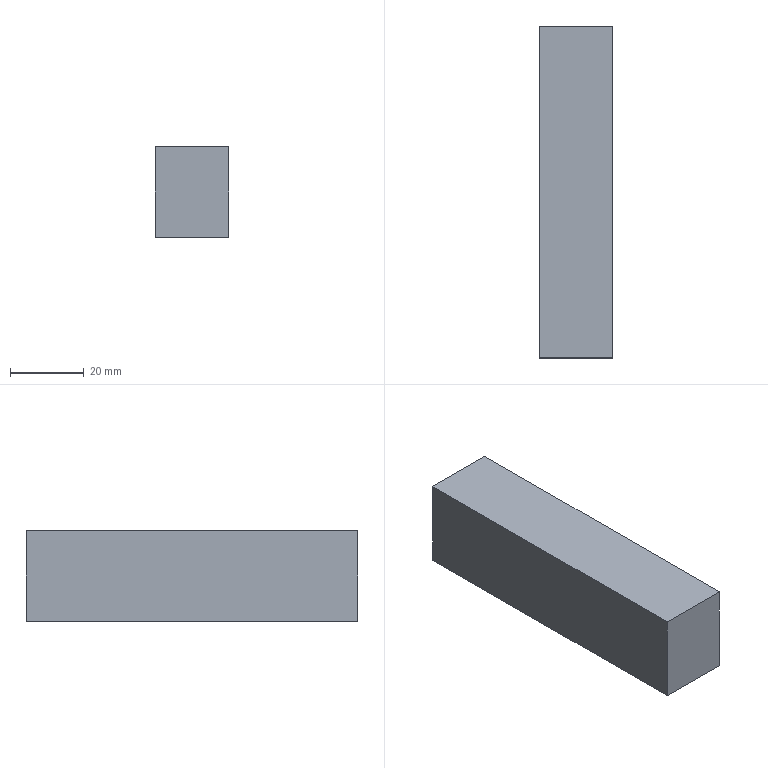Part | SolidWorks | features Extrusion 1 | 1 solid | 6 faces | box 20 x 90 x 24.5 mm | volume 44100 mm3 | plane 6
STEP:
#1=CARTESIAN_POINT('',(0.,45.,0.));
#2=VERTEX_POINT('',#1);
#3=CARTESIAN_POINT('',(0.,-45.,0.));
#4=VERTEX_POINT('',#3);
#5=CARTESIAN_POINT('',(0.,45.,0.));
#6=DIRECTION('',(0.,-1.,0.));
#7=VECTOR('',#6,1000.);
#8=LINE('',#5,#7);
#9=EDGE_CURVE('',#2,#4,#8,.T.);
#10=ORIENTED_EDGE('',*,*,#9,.T.);
#11=CARTESIAN_POINT('',(0.,-45.,24.5));
#12=VERTEX_POINT('',#11);
#13=CARTESIAN_POINT('',(0.,-45.,24.5));
#14=DIRECTION('',(0.,0.,-1.));
#15=VECTOR('',#14,1000.);
#16=LINE('',#13,#15);
#17=EDGE_CURVE('',#12,#4,#16,.T.);
#18=ORIENTED_EDGE('',*,*,#17,.F.);
#19=CARTESIAN_POINT('',(0.,45.,24.5));
#20=VERTEX_POINT('',#19);
#21=CARTESIAN_POINT('',(0.,45.,24.5));
#22=DIRECTION('',(0.,-1.,0.));
#23=VECTOR('',#22,1000.);
#24=LINE('',#21,#23);
#25=EDGE_CURVE('',#20,#12,#24,.T.);
#26=ORIENTED_EDGE('',*,*,#25,.F.);
#27=CARTESIAN_POINT('',(0.,45.,24.5));
#28=DIRECTION('',(0.,0.,-1.));
#29=VECTOR('',#28,1000.);
#30=LINE('',#27,#29);
#31=EDGE_CURVE('',#20,#2,#30,.T.);
#32=ORIENTED_EDGE('',*,*,#31,.T.);
#33=EDGE_LOOP('',(#10,#18,#26,#32));
#34=FACE_OUTER_BOUND('',#33,.T.);
#35=CARTESIAN_POINT('',(0.,45.,24.5));
#36=DIRECTION('',(1.,0.,0.));
#37=DIRECTION('',(0.,0.,-1.));
#38=AXIS2_PLACEMENT_3D('',#35,#36,#37);
#39=PLANE('',#38);
#40=ADVANCED_FACE('',(#34),#39,.F.);
#41=CARTESIAN_POINT('',(20.,-45.,0.));
#42=VERTEX_POINT('',#41);
#43=CARTESIAN_POINT('',(0.,-45.,0.));
#44=DIRECTION('',(1.,0.,0.));
#45=VECTOR('',#44,1000.);
#46=LINE('',#43,#45);
#47=EDGE_CURVE('',#4,#42,#46,.T.);
#48=ORIENTED_EDGE('',*,*,#47,.T.);
#49=CARTESIAN_POINT('',(20.,-45.,24.5));
#50=VERTEX_POINT('',#49);
#51=CARTESIAN_POINT('',(20.,-45.,24.5));
#52=DIRECTION('',(0.,0.,-1.));
#53=VECTOR('',#52,1000.);
#54=LINE('',#51,#53);
#55=EDGE_CURVE('',#50,#42,#54,.T.);
#56=ORIENTED_EDGE('',*,*,#55,.F.);
#57=CARTESIAN_POINT('',(0.,-45.,24.5));
#58=DIRECTION('',(1.,0.,0.));
#59=VECTOR('',#58,1000.);
#60=LINE('',#57,#59);
#61=EDGE_CURVE('',#12,#50,#60,.T.);
#62=ORIENTED_EDGE('',*,*,#61,.F.);
#63=ORIENTED_EDGE('',*,*,#17,.T.);
#64=EDGE_LOOP('',(#48,#56,#62,#63));
#65=FACE_OUTER_BOUND('',#64,.T.);
#66=CARTESIAN_POINT('',(0.,-45.,24.5));
#67=DIRECTION('',(0.,1.,0.));
#68=DIRECTION('',(0.,0.,1.));
#69=AXIS2_PLACEMENT_3D('',#66,#67,#68);
#70=PLANE('',#69);
#71=ADVANCED_FACE('',(#65),#70,.F.);
#72=CARTESIAN_POINT('',(20.,45.,0.));
#73=VERTEX_POINT('',#72);
#74=CARTESIAN_POINT('',(20.,45.,0.));
#75=DIRECTION('',(0.,1.,0.));
#76=VECTOR('',#75,1000.);
#77=LINE('',#74,#76);
#78=EDGE_CURVE('',#42,#73,#77,.T.);
#79=ORIENTED_EDGE('',*,*,#78,.T.);
#80=CARTESIAN_POINT('',(20.,45.,24.5));
#81=VERTEX_POINT('',#80);
#82=CARTESIAN_POINT('',(20.,45.,24.5));
#83=DIRECTION('',(0.,0.,-1.));
#84=VECTOR('',#83,1000.);
#85=LINE('',#82,#84);
#86=EDGE_CURVE('',#81,#73,#85,.T.);
#87=ORIENTED_EDGE('',*,*,#86,.F.);
#88=CARTESIAN_POINT('',(20.,45.,24.5));
#89=DIRECTION('',(0.,1.,0.));
#90=VECTOR('',#89,1000.);
#91=LINE('',#88,#90);
#92=EDGE_CURVE('',#50,#81,#91,.T.);
#93=ORIENTED_EDGE('',*,*,#92,.F.);
#94=ORIENTED_EDGE('',*,*,#55,.T.);
#95=EDGE_LOOP('',(#79,#87,#93,#94));
#96=FACE_OUTER_BOUND('',#95,.T.);
#97=CARTESIAN_POINT('',(20.,45.,24.5));
#98=DIRECTION('',(-1.,0.,0.));
#99=DIRECTION('',(0.,-1.,0.));
#100=AXIS2_PLACEMENT_3D('',#97,#98,#99);
#101=PLANE('',#100);
#102=ADVANCED_FACE('',(#96),#101,.F.);
#103=CARTESIAN_POINT('',(0.,45.,0.));
#104=DIRECTION('',(-1.,0.,0.));
#105=VECTOR('',#104,1000.);
#106=LINE('',#103,#105);
#107=EDGE_CURVE('',#73,#2,#106,.T.);
#108=ORIENTED_EDGE('',*,*,#107,.T.);
#109=ORIENTED_EDGE('',*,*,#31,.F.);
#110=CARTESIAN_POINT('',(0.,45.,24.5));
#111=DIRECTION('',(-1.,0.,0.));
#112=VECTOR('',#111,1000.);
#113=LINE('',#110,#112);
#114=EDGE_CURVE('',#81,#20,#113,.T.);
#115=ORIENTED_EDGE('',*,*,#114,.F.);
#116=ORIENTED_EDGE('',*,*,#86,.T.);
#117=EDGE_LOOP('',(#108,#109,#115,#116));
#118=FACE_OUTER_BOUND('',#117,.T.);
#119=CARTESIAN_POINT('',(0.,45.,24.5));
#120=DIRECTION('',(0.,-1.,0.));
#121=DIRECTION('',(0.,0.,-1.));
#122=AXIS2_PLACEMENT_3D('',#119,#120,#121);
#123=PLANE('',#122);
#124=ADVANCED_FACE('',(#118),#123,.F.);
#125=ORIENTED_EDGE('',*,*,#25,.T.);
#126=ORIENTED_EDGE('',*,*,#61,.T.);
#127=ORIENTED_EDGE('',*,*,#92,.T.);
#128=ORIENTED_EDGE('',*,*,#114,.T.);
#129=EDGE_LOOP('',(#125,#126,#127,#128));
#130=FACE_OUTER_BOUND('',#129,.T.);
#131=CARTESIAN_POINT('',(0.,0.,24.5));
#132=DIRECTION('',(0.,0.,1.));
#133=DIRECTION('',(1.,0.,0.));
#134=AXIS2_PLACEMENT_3D('',#131,#132,#133);
#135=PLANE('',#134);
#136=ADVANCED_FACE('',(#130),#135,.T.);
#137=ORIENTED_EDGE('',*,*,#9,.F.);
#138=ORIENTED_EDGE('',*,*,#107,.F.);
#139=ORIENTED_EDGE('',*,*,#78,.F.);
#140=ORIENTED_EDGE('',*,*,#47,.F.);
#141=EDGE_LOOP('',(#137,#138,#139,#140));
#142=FACE_OUTER_BOUND('',#141,.T.);
#143=CARTESIAN_POINT('',(0.,0.,0.));
#144=DIRECTION('',(0.,0.,1.));
#145=DIRECTION('',(1.,0.,0.));
#146=AXIS2_PLACEMENT_3D('',#143,#144,#145);
#147=PLANE('',#146);
#148=ADVANCED_FACE('',(#142),#147,.F.);
#149=CLOSED_SHELL('',(#40,#71,#102,#124,#136,#148));
#150=MANIFOLD_SOLID_BREP('',#149);
#151=CARTESIAN_POINT('',(0.,0.,0.));
#152=DIRECTION('',(0.,0.,1.));
#153=DIRECTION('',(1.,0.,0.));
#154=AXIS2_PLACEMENT_3D('',#151,#152,#153);
#155=(LENGTH_UNIT()NAMED_UNIT(*)SI_UNIT(.MILLI.,.METRE.));
#156=UNCERTAINTY_MEASURE_WITH_UNIT(LENGTH_MEASURE(0.00001),#155,'','');
#157=(NAMED_UNIT(*)PLANE_ANGLE_UNIT()SI_UNIT($,.RADIAN.));
#158=(NAMED_UNIT(*)SI_UNIT($,.STERADIAN.)SOLID_ANGLE_UNIT());
#159=(GEOMETRIC_REPRESENTATION_CONTEXT(3)GLOBAL_UNCERTAINTY_ASSIGNED_CONTEXT((#156))GLOBAL_UNIT_ASSIGNED_CONTEXT((#155,#157,#158))REPRESENTATION_CONTEXT('',''));
#160=ADVANCED_BREP_SHAPE_REPRESENTATION('',(#150,#154),#159);